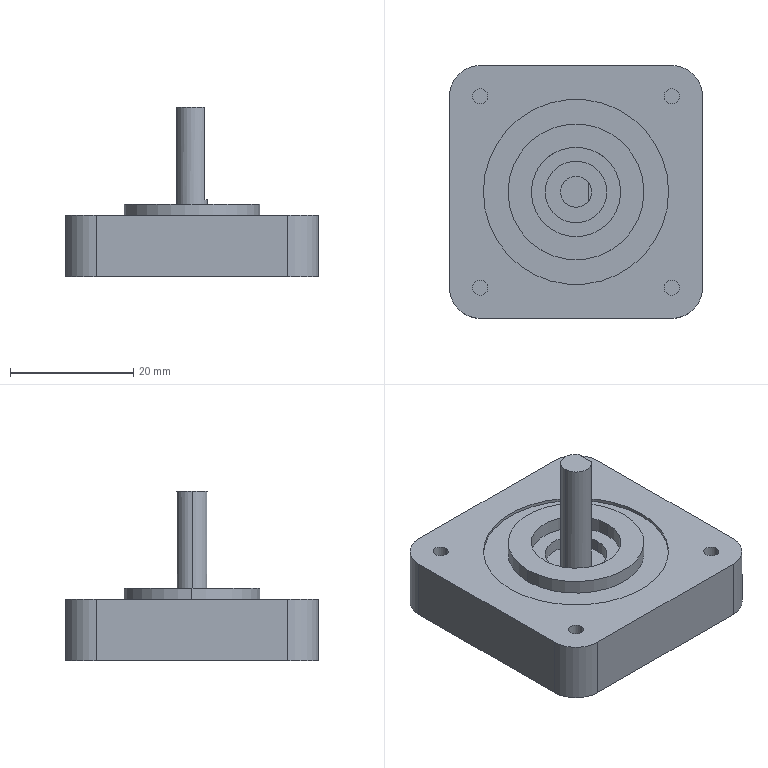Part | SolidWorks | features BaseBody 1 | 1 solid | 39 faces | box 41 x 41 x 27.5 mm | volume 16881 mm3 | cylinder 22 | plane 17 | commonest cylinder face diameters 2.459 x8 10 x6 5 x2 14.5 x2 22 x2 30 x2
STEP:
#1=CARTESIAN_POINT('',(-2.739,-8.029,6.));
#2=VERTEX_POINT('',#1);
#3=CARTESIAN_POINT('',(-0.2798,-8.029,6.));
#4=VERTEX_POINT('',#3);
#5=CARTESIAN_POINT('',(-1.509,-8.029,6.));
#6=DIRECTION('',(0.,0.,1.));
#7=DIRECTION('',(1.,0.,0.));
#8=AXIS2_PLACEMENT_3D('',#5,#6,#7);
#9=CIRCLE('',#8,1.23);
#10=EDGE_CURVE('',#2,#4,#9,.T.);
#11=ORIENTED_EDGE('',*,*,#10,.F.);
#12=CARTESIAN_POINT('',(-2.739,-8.029,10.));
#13=VERTEX_POINT('',#12);
#14=CARTESIAN_POINT('',(-2.739,-8.029,8.));
#15=DIRECTION('',(0.,0.,1.));
#16=VECTOR('',#15,1000.);
#17=LINE('',#14,#16);
#18=EDGE_CURVE('',#2,#13,#17,.T.);
#19=ORIENTED_EDGE('',*,*,#18,.T.);
#20=CARTESIAN_POINT('',(-0.2798,-8.029,10.));
#21=VERTEX_POINT('',#20);
#22=CARTESIAN_POINT('',(-1.509,-8.029,10.));
#23=DIRECTION('',(0.,0.,-1.));
#24=DIRECTION('',(1.,0.,0.));
#25=AXIS2_PLACEMENT_3D('',#22,#23,#24);
#26=CIRCLE('',#25,1.23);
#27=EDGE_CURVE('',#21,#13,#26,.T.);
#28=ORIENTED_EDGE('',*,*,#27,.F.);
#29=CARTESIAN_POINT('',(-0.2798,-8.029,8.));
#30=DIRECTION('',(0.,0.,1.));
#31=VECTOR('',#30,1000.);
#32=LINE('',#29,#31);
#33=EDGE_CURVE('',#4,#21,#32,.T.);
#34=ORIENTED_EDGE('',*,*,#33,.F.);
#35=EDGE_LOOP('',(#11,#19,#28,#34));
#36=FACE_OUTER_BOUND('',#35,.T.);
#37=CARTESIAN_POINT('',(-1.509,-8.029,8.));
#38=DIRECTION('',(0.,0.,1.));
#39=DIRECTION('',(1.,0.,0.));
#40=AXIS2_PLACEMENT_3D('',#37,#38,#39);
#41=CYLINDRICAL_SURFACE('',#40,1.23);
#42=ADVANCED_FACE('',(#36),#41,.F.);
#43=CARTESIAN_POINT('',(-33.739,-8.029,6.));
#44=VERTEX_POINT('',#43);
#45=CARTESIAN_POINT('',(-31.28,-8.029,6.));
#46=VERTEX_POINT('',#45);
#47=CARTESIAN_POINT('',(-32.509,-8.029,6.));
#48=DIRECTION('',(0.,0.,1.));
#49=DIRECTION('',(1.,0.,0.));
#50=AXIS2_PLACEMENT_3D('',#47,#48,#49);
#51=CIRCLE('',#50,1.23);
#52=EDGE_CURVE('',#44,#46,#51,.T.);
#53=ORIENTED_EDGE('',*,*,#52,.F.);
#54=CARTESIAN_POINT('',(-33.739,-8.029,10.));
#55=VERTEX_POINT('',#54);
#56=CARTESIAN_POINT('',(-33.739,-8.029,8.));
#57=DIRECTION('',(0.,0.,1.));
#58=VECTOR('',#57,1000.);
#59=LINE('',#56,#58);
#60=EDGE_CURVE('',#44,#55,#59,.T.);
#61=ORIENTED_EDGE('',*,*,#60,.T.);
#62=CARTESIAN_POINT('',(-31.28,-8.029,10.));
#63=VERTEX_POINT('',#62);
#64=CARTESIAN_POINT('',(-32.509,-8.029,10.));
#65=DIRECTION('',(0.,0.,-1.));
#66=DIRECTION('',(1.,0.,0.));
#67=AXIS2_PLACEMENT_3D('',#64,#65,#66);
#68=CIRCLE('',#67,1.23);
#69=EDGE_CURVE('',#63,#55,#68,.T.);
#70=ORIENTED_EDGE('',*,*,#69,.F.);
#71=CARTESIAN_POINT('',(-31.28,-8.029,8.));
#72=DIRECTION('',(0.,0.,1.));
#73=VECTOR('',#72,1000.);
#74=LINE('',#71,#73);
#75=EDGE_CURVE('',#46,#63,#74,.T.);
#76=ORIENTED_EDGE('',*,*,#75,.F.);
#77=EDGE_LOOP('',(#53,#61,#70,#76));
#78=FACE_OUTER_BOUND('',#77,.T.);
#79=CARTESIAN_POINT('',(-32.509,-8.029,8.));
#80=DIRECTION('',(0.,0.,1.));
#81=DIRECTION('',(1.,0.,0.));
#82=AXIS2_PLACEMENT_3D('',#79,#80,#81);
#83=CYLINDRICAL_SURFACE('',#82,1.23);
#84=ADVANCED_FACE('',(#78),#83,.F.);
#85=CARTESIAN_POINT('',(-33.739,22.971,6.));
#86=VERTEX_POINT('',#85);
#87=CARTESIAN_POINT('',(-31.28,22.971,6.));
#88=VERTEX_POINT('',#87);
#89=CARTESIAN_POINT('',(-32.509,22.971,6.));
#90=DIRECTION('',(0.,0.,1.));
#91=DIRECTION('',(1.,0.,0.));
#92=AXIS2_PLACEMENT_3D('',#89,#90,#91);
#93=CIRCLE('',#92,1.23);
#94=EDGE_CURVE('',#86,#88,#93,.T.);
#95=ORIENTED_EDGE('',*,*,#94,.F.);
#96=CARTESIAN_POINT('',(-33.739,22.971,10.));
#97=VERTEX_POINT('',#96);
#98=CARTESIAN_POINT('',(-33.739,22.971,8.));
#99=DIRECTION('',(0.,0.,1.));
#100=VECTOR('',#99,1000.);
#101=LINE('',#98,#100);
#102=EDGE_CURVE('',#86,#97,#101,.T.);
#103=ORIENTED_EDGE('',*,*,#102,.T.);
#104=CARTESIAN_POINT('',(-31.28,22.971,10.));
#105=VERTEX_POINT('',#104);
#106=CARTESIAN_POINT('',(-32.509,22.971,10.));
#107=DIRECTION('',(0.,0.,-1.));
#108=DIRECTION('',(1.,0.,0.));
#109=AXIS2_PLACEMENT_3D('',#106,#107,#108);
#110=CIRCLE('',#109,1.23);
#111=EDGE_CURVE('',#105,#97,#110,.T.);
#112=ORIENTED_EDGE('',*,*,#111,.F.);
#113=CARTESIAN_POINT('',(-31.28,22.971,8.));
#114=DIRECTION('',(0.,0.,1.));
#115=VECTOR('',#114,1000.);
#116=LINE('',#113,#115);
#117=EDGE_CURVE('',#88,#105,#116,.T.);
#118=ORIENTED_EDGE('',*,*,#117,.F.);
#119=EDGE_LOOP('',(#95,#103,#112,#118));
#120=FACE_OUTER_BOUND('',#119,.T.);
#121=CARTESIAN_POINT('',(-32.509,22.971,8.));
#122=DIRECTION('',(0.,0.,1.));
#123=DIRECTION('',(1.,0.,0.));
#124=AXIS2_PLACEMENT_3D('',#121,#122,#123);
#125=CYLINDRICAL_SURFACE('',#124,1.23);
#126=ADVANCED_FACE('',(#120),#125,.F.);
#127=CARTESIAN_POINT('',(-2.739,22.971,6.));
#128=VERTEX_POINT('',#127);
#129=CARTESIAN_POINT('',(-0.2798,22.971,6.));
#130=VERTEX_POINT('',#129);
#131=CARTESIAN_POINT('',(-1.509,22.971,6.));
#132=DIRECTION('',(0.,0.,1.));
#133=DIRECTION('',(1.,0.,0.));
#134=AXIS2_PLACEMENT_3D('',#131,#132,#133);
#135=CIRCLE('',#134,1.23);
#136=EDGE_CURVE('',#128,#130,#135,.T.);
#137=ORIENTED_EDGE('',*,*,#136,.F.);
#138=CARTESIAN_POINT('',(-2.739,22.971,10.));
#139=VERTEX_POINT('',#138);
#140=CARTESIAN_POINT('',(-2.739,22.971,8.));
#141=DIRECTION('',(0.,0.,1.));
#142=VECTOR('',#141,1000.);
#143=LINE('',#140,#142);
#144=EDGE_CURVE('',#128,#139,#143,.T.);
#145=ORIENTED_EDGE('',*,*,#144,.T.);
#146=CARTESIAN_POINT('',(-0.2798,22.971,10.));
#147=VERTEX_POINT('',#146);
#148=CARTESIAN_POINT('',(-1.509,22.971,10.));
#149=DIRECTION('',(0.,0.,-1.));
#150=DIRECTION('',(1.,0.,0.));
#151=AXIS2_PLACEMENT_3D('',#148,#149,#150);
#152=CIRCLE('',#151,1.23);
#153=EDGE_CURVE('',#147,#139,#152,.T.);
#154=ORIENTED_EDGE('',*,*,#153,.F.);
#155=CARTESIAN_POINT('',(-0.2798,22.971,8.));
#156=DIRECTION('',(0.,0.,1.));
#157=VECTOR('',#156,1000.);
#158=LINE('',#155,#157);
#159=EDGE_CURVE('',#130,#147,#158,.T.);
#160=ORIENTED_EDGE('',*,*,#159,.F.);
#161=EDGE_LOOP('',(#137,#145,#154,#160));
#162=FACE_OUTER_BOUND('',#161,.T.);
#163=CARTESIAN_POINT('',(-1.509,22.971,8.));
#164=DIRECTION('',(0.,0.,1.));
#165=DIRECTION('',(1.,0.,0.));
#166=AXIS2_PLACEMENT_3D('',#163,#164,#165);
#167=CYLINDRICAL_SURFACE('',#166,1.23);
#168=ADVANCED_FACE('',(#162),#167,.F.);
#169=CARTESIAN_POINT('',(-2.009,7.471,10.));
#170=VERTEX_POINT('',#169);
#171=CARTESIAN_POINT('',(-32.009,7.471,10.));
#172=VERTEX_POINT('',#171);
#173=CARTESIAN_POINT('',(-17.009,7.471,10.));
#174=DIRECTION('',(0.,0.,-1.));
#175=DIRECTION('',(-1.,0.,0.));
#176=AXIS2_PLACEMENT_3D('',#173,#174,#175);
#177=CIRCLE('',#176,15.);
#178=EDGE_CURVE('',#170,#172,#177,.T.);
#179=ORIENTED_EDGE('',*,*,#178,.F.);
#180=CARTESIAN_POINT('',(-2.009,7.471,9.5));
#181=VERTEX_POINT('',#180);
#182=CARTESIAN_POINT('',(-2.009,7.471,10.));
#183=DIRECTION('',(0.,0.,-1.));
#184=VECTOR('',#183,1000.);
#185=LINE('',#182,#184);
#186=EDGE_CURVE('',#170,#181,#185,.T.);
#187=ORIENTED_EDGE('',*,*,#186,.T.);
#188=CARTESIAN_POINT('',(-32.009,7.471,9.5));
#189=VERTEX_POINT('',#188);
#190=CARTESIAN_POINT('',(-17.009,7.471,9.5));
#191=DIRECTION('',(0.,0.,1.));
#192=DIRECTION('',(-1.,0.,0.));
#193=AXIS2_PLACEMENT_3D('',#190,#191,#192);
#194=CIRCLE('',#193,15.);
#195=EDGE_CURVE('',#189,#181,#194,.T.);
#196=ORIENTED_EDGE('',*,*,#195,.F.);
#197=CARTESIAN_POINT('',(-32.009,7.471,10.));
#198=DIRECTION('',(0.,0.,-1.));
#199=VECTOR('',#198,1000.);
#200=LINE('',#197,#199);
#201=EDGE_CURVE('',#172,#189,#200,.T.);
#202=ORIENTED_EDGE('',*,*,#201,.F.);
#203=EDGE_LOOP('',(#179,#187,#196,#202));
#204=FACE_OUTER_BOUND('',#203,.T.);
#205=CARTESIAN_POINT('',(-17.009,7.471,10.));
#206=DIRECTION('',(0.,0.,-1.));
#207=DIRECTION('',(-1.,0.,0.));
#208=AXIS2_PLACEMENT_3D('',#205,#206,#207);
#209=CYLINDRICAL_SURFACE('',#208,15.);
#210=ADVANCED_FACE('',(#204),#209,.F.);
#211=CARTESIAN_POINT('',(-6.009,7.471,9.5));
#212=VERTEX_POINT('',#211);
#213=CARTESIAN_POINT('',(-28.009,7.471,9.5));
#214=VERTEX_POINT('',#213);
#215=CARTESIAN_POINT('',(-17.009,7.471,9.5));
#216=DIRECTION('',(0.,0.,1.));
#217=DIRECTION('',(1.,0.,0.));
#218=AXIS2_PLACEMENT_3D('',#215,#216,#217);
#219=CIRCLE('',#218,11.);
#220=EDGE_CURVE('',#212,#214,#219,.T.);
#221=ORIENTED_EDGE('',*,*,#220,.T.);
#222=CARTESIAN_POINT('',(-28.009,7.471,11.8));
#223=VERTEX_POINT('',#222);
#224=CARTESIAN_POINT('',(-28.009,7.471,9.5));
#225=DIRECTION('',(0.,0.,1.));
#226=VECTOR('',#225,1000.);
#227=LINE('',#224,#226);
#228=EDGE_CURVE('',#214,#223,#227,.T.);
#229=ORIENTED_EDGE('',*,*,#228,.T.);
#230=CARTESIAN_POINT('',(-6.009,7.471,11.8));
#231=VERTEX_POINT('',#230);
#232=CARTESIAN_POINT('',(-17.009,7.471,11.8));
#233=DIRECTION('',(0.,0.,-1.));
#234=DIRECTION('',(1.,0.,0.));
#235=AXIS2_PLACEMENT_3D('',#232,#233,#234);
#236=CIRCLE('',#235,11.);
#237=EDGE_CURVE('',#223,#231,#236,.T.);
#238=ORIENTED_EDGE('',*,*,#237,.T.);
#239=CARTESIAN_POINT('',(-6.009,7.471,9.5));
#240=DIRECTION('',(0.,0.,1.));
#241=VECTOR('',#240,1000.);
#242=LINE('',#239,#241);
#243=EDGE_CURVE('',#212,#231,#242,.T.);
#244=ORIENTED_EDGE('',*,*,#243,.F.);
#245=EDGE_LOOP('',(#221,#229,#238,#244));
#246=FACE_OUTER_BOUND('',#245,.T.);
#247=CARTESIAN_POINT('',(-17.009,7.471,9.5));
#248=DIRECTION('',(0.,0.,1.));
#249=DIRECTION('',(1.,0.,0.));
#250=AXIS2_PLACEMENT_3D('',#247,#248,#249);
#251=CYLINDRICAL_SURFACE('',#250,11.);
#252=ADVANCED_FACE('',(#246),#251,.T.);
#253=CARTESIAN_POINT('',(-24.259,7.471,9.5));
#254=VERTEX_POINT('',#253);
#255=CARTESIAN_POINT('',(-9.759,7.471,9.5));
#256=VERTEX_POINT('',#255);
#257=CARTESIAN_POINT('',(-17.009,7.471,9.5));
#258=DIRECTION('',(0.,0.,1.));
#259=DIRECTION('',(1.,0.,0.));
#260=AXIS2_PLACEMENT_3D('',#257,#258,#259);
#261=CIRCLE('',#260,7.25);
#262=EDGE_CURVE('',#254,#256,#261,.T.);
#263=ORIENTED_EDGE('',*,*,#262,.F.);
#264=CARTESIAN_POINT('',(-24.259,7.471,11.8));
#265=VERTEX_POINT('',#264);
#266=CARTESIAN_POINT('',(-24.259,7.471,10.65));
#267=DIRECTION('',(0.,0.,1.));
#268=VECTOR('',#267,1000.);
#269=LINE('',#266,#268);
#270=EDGE_CURVE('',#254,#265,#269,.T.);
#271=ORIENTED_EDGE('',*,*,#270,.T.);
#272=CARTESIAN_POINT('',(-9.759,7.471,11.8));
#273=VERTEX_POINT('',#272);
#274=CARTESIAN_POINT('',(-17.009,7.471,11.8));
#275=DIRECTION('',(0.,0.,1.));
#276=DIRECTION('',(1.,0.,0.));
#277=AXIS2_PLACEMENT_3D('',#274,#275,#276);
#278=CIRCLE('',#277,7.25);
#279=EDGE_CURVE('',#265,#273,#278,.T.);
#280=ORIENTED_EDGE('',*,*,#279,.T.);
#281=CARTESIAN_POINT('',(-9.759,7.471,10.65));
#282=DIRECTION('',(0.,0.,1.));
#283=VECTOR('',#282,1000.);
#284=LINE('',#281,#283);
#285=EDGE_CURVE('',#256,#273,#284,.T.);
#286=ORIENTED_EDGE('',*,*,#285,.F.);
#287=EDGE_LOOP('',(#263,#271,#280,#286));
#288=FACE_OUTER_BOUND('',#287,.T.);
#289=CARTESIAN_POINT('',(-17.009,7.471,10.65));
#290=DIRECTION('',(0.,0.,1.));
#291=DIRECTION('',(1.,0.,0.));
#292=AXIS2_PLACEMENT_3D('',#289,#290,#291);
#293=CYLINDRICAL_SURFACE('',#292,7.25);
#294=ADVANCED_FACE('',(#288),#293,.F.);
#295=CARTESIAN_POINT('',(-22.009,7.471,7.5));
#296=VERTEX_POINT('',#295);
#297=CARTESIAN_POINT('',(-12.009,7.471,7.5));
#298=VERTEX_POINT('',#297);
#299=CARTESIAN_POINT('',(-17.009,7.471,7.5));
#300=DIRECTION('',(0.,0.,1.));
#301=DIRECTION('',(1.,0.,0.));
#302=AXIS2_PLACEMENT_3D('',#299,#300,#301);
#303=CIRCLE('',#302,5.);
#304=EDGE_CURVE('',#296,#298,#303,.T.);
#305=ORIENTED_EDGE('',*,*,#304,.F.);
#306=CARTESIAN_POINT('',(-22.009,7.471,9.5));
#307=VERTEX_POINT('',#306);
#308=CARTESIAN_POINT('',(-22.009,7.471,8.75));
#309=DIRECTION('',(0.,0.,1.));
#310=VECTOR('',#309,1000.);
#311=LINE('',#308,#310);
#312=EDGE_CURVE('',#296,#307,#311,.T.);
#313=ORIENTED_EDGE('',*,*,#312,.T.);
#314=CARTESIAN_POINT('',(-12.009,7.471,9.5));
#315=VERTEX_POINT('',#314);
#316=CARTESIAN_POINT('',(-17.009,7.471,9.5));
#317=DIRECTION('',(0.,0.,-1.));
#318=DIRECTION('',(1.,0.,0.));
#319=AXIS2_PLACEMENT_3D('',#316,#317,#318);
#320=CIRCLE('',#319,5.);
#321=EDGE_CURVE('',#315,#307,#320,.T.);
#322=ORIENTED_EDGE('',*,*,#321,.F.);
#323=CARTESIAN_POINT('',(-12.009,7.471,8.75));
#324=DIRECTION('',(0.,0.,1.));
#325=VECTOR('',#324,1000.);
#326=LINE('',#323,#325);
#327=EDGE_CURVE('',#298,#315,#326,.T.);
#328=ORIENTED_EDGE('',*,*,#327,.F.);
#329=EDGE_LOOP('',(#305,#313,#322,#328));
#330=FACE_OUTER_BOUND('',#329,.T.);
#331=CARTESIAN_POINT('',(-17.009,7.471,8.75));
#332=DIRECTION('',(0.,0.,1.));
#333=DIRECTION('',(1.,0.,0.));
#334=AXIS2_PLACEMENT_3D('',#331,#332,#333);
#335=CYLINDRICAL_SURFACE('',#334,5.);
#336=ADVANCED_FACE('',(#330),#335,.F.);
#337=CARTESIAN_POINT('',(-19.509,7.471,7.5));
#338=VERTEX_POINT('',#337);
#339=CARTESIAN_POINT('',(-14.509,7.471,7.5));
#340=VERTEX_POINT('',#339);
#341=CARTESIAN_POINT('',(-17.009,7.471,7.5));
#342=DIRECTION('',(0.,0.,-1.));
#343=DIRECTION('',(1.,0.,0.));
#344=AXIS2_PLACEMENT_3D('',#341,#342,#343);
#345=CIRCLE('',#344,2.5);
#346=EDGE_CURVE('',#338,#340,#345,.T.);
#347=ORIENTED_EDGE('',*,*,#346,.F.);
#348=CARTESIAN_POINT('',(-19.509,7.471,27.5));
#349=VERTEX_POINT('',#348);
#350=CARTESIAN_POINT('',(-19.509,7.471,7.5));
#351=DIRECTION('',(0.,0.,1.));
#352=VECTOR('',#351,1000.);
#353=LINE('',#350,#352);
#354=EDGE_CURVE('',#338,#349,#353,.T.);
#355=ORIENTED_EDGE('',*,*,#354,.T.);
#356=CARTESIAN_POINT('',(-15.009,8.971,27.5));
#357=VERTEX_POINT('',#356);
#358=CARTESIAN_POINT('',(-17.009,7.471,27.5));
#359=DIRECTION('',(0.,0.,-1.));
#360=DIRECTION('',(1.,0.,0.));
#361=AXIS2_PLACEMENT_3D('',#358,#359,#360);
#362=CIRCLE('',#361,2.5);
#363=EDGE_CURVE('',#349,#357,#362,.T.);
#364=ORIENTED_EDGE('',*,*,#363,.T.);
#365=CARTESIAN_POINT('',(-15.009,8.971,12.5));
#366=VERTEX_POINT('',#365);
#367=CARTESIAN_POINT('',(-15.009,8.971,7.5));
#368=DIRECTION('',(0.,0.,-1.));
#369=VECTOR('',#368,1000.);
#370=LINE('',#367,#369);
#371=EDGE_CURVE('',#357,#366,#370,.T.);
#372=ORIENTED_EDGE('',*,*,#371,.T.);
#373=CARTESIAN_POINT('',(-14.509,7.471,12.5));
#374=VERTEX_POINT('',#373);
#375=CARTESIAN_POINT('',(-17.009,7.471,12.5));
#376=DIRECTION('',(0.,0.,-1.));
#377=DIRECTION('',(1.,0.,0.));
#378=AXIS2_PLACEMENT_3D('',#375,#376,#377);
#379=CIRCLE('',#378,2.5);
#380=EDGE_CURVE('',#366,#374,#379,.T.);
#381=ORIENTED_EDGE('',*,*,#380,.T.);
#382=CARTESIAN_POINT('',(-14.509,7.471,7.5));
#383=DIRECTION('',(0.,0.,1.));
#384=VECTOR('',#383,1000.);
#385=LINE('',#382,#384);
#386=EDGE_CURVE('',#340,#374,#385,.T.);
#387=ORIENTED_EDGE('',*,*,#386,.F.);
#388=EDGE_LOOP('',(#347,#355,#364,#372,#381,#387));
#389=FACE_OUTER_BOUND('',#388,.T.);
#390=CARTESIAN_POINT('',(-17.009,7.471,7.5));
#391=DIRECTION('',(0.,0.,1.));
#392=DIRECTION('',(1.,0.,0.));
#393=AXIS2_PLACEMENT_3D('',#390,#391,#392);
#394=CYLINDRICAL_SURFACE('',#393,2.5);
#395=ADVANCED_FACE('',(#389),#394,.T.);
#396=CARTESIAN_POINT('',(-37.509,22.971,0.));
#397=VERTEX_POINT('',#396);
#398=CARTESIAN_POINT('',(-37.509,-8.029,0.));
#399=VERTEX_POINT('',#398);
#400=CARTESIAN_POINT('',(-37.509,7.471,0.));
#401=DIRECTION('',(0.,-1.,0.));
#402=VECTOR('',#401,1000.);
#403=LINE('',#400,#402);
#404=EDGE_CURVE('',#397,#399,#403,.T.);
#405=ORIENTED_EDGE('',*,*,#404,.F.);
#406=CARTESIAN_POINT('',(-32.509,27.971,0.));
#407=VERTEX_POINT('',#406);
#408=CARTESIAN_POINT('',(-32.509,22.971,0.));
#409=DIRECTION('',(0.,0.,1.));
#410=DIRECTION('',(1.,0.,0.));
#411=AXIS2_PLACEMENT_3D('',#408,#409,#410);
#412=CIRCLE('',#411,5.);
#413=EDGE_CURVE('',#407,#397,#412,.T.);
#414=ORIENTED_EDGE('',*,*,#413,.F.);
#415=CARTESIAN_POINT('',(-1.509,27.971,0.));
#416=VERTEX_POINT('',#415);
#417=CARTESIAN_POINT('',(-17.009,27.971,0.));
#418=DIRECTION('',(-1.,0.,0.));
#419=VECTOR('',#418,1000.);
#420=LINE('',#417,#419);
#421=EDGE_CURVE('',#416,#407,#420,.T.);
#422=ORIENTED_EDGE('',*,*,#421,.F.);
#423=CARTESIAN_POINT('',(3.491,22.971,0.));
#424=VERTEX_POINT('',#423);
#425=CARTESIAN_POINT('',(-1.509,22.971,0.));
#426=DIRECTION('',(0.,0.,1.));
#427=DIRECTION('',(1.,0.,0.));
#428=AXIS2_PLACEMENT_3D('',#425,#426,#427);
#429=CIRCLE('',#428,5.);
#430=EDGE_CURVE('',#424,#416,#429,.T.);
#431=ORIENTED_EDGE('',*,*,#430,.F.);
#432=CARTESIAN_POINT('',(3.491,-8.029,0.));
#433=VERTEX_POINT('',#432);
#434=CARTESIAN_POINT('',(3.491,7.471,0.));
#435=DIRECTION('',(0.,1.,0.));
#436=VECTOR('',#435,1000.);
#437=LINE('',#434,#436);
#438=EDGE_CURVE('',#433,#424,#437,.T.);
#439=ORIENTED_EDGE('',*,*,#438,.F.);
#440=CARTESIAN_POINT('',(-1.509,-13.029,0.));
#441=VERTEX_POINT('',#440);
#442=CARTESIAN_POINT('',(-1.509,-8.029,0.));
#443=DIRECTION('',(0.,0.,1.));
#444=DIRECTION('',(1.,0.,0.));
#445=AXIS2_PLACEMENT_3D('',#442,#443,#444);
#446=CIRCLE('',#445,5.);
#447=EDGE_CURVE('',#441,#433,#446,.T.);
#448=ORIENTED_EDGE('',*,*,#447,.F.);
#449=CARTESIAN_POINT('',(-32.509,-13.029,0.));
#450=VERTEX_POINT('',#449);
#451=CARTESIAN_POINT('',(-17.009,-13.029,0.));
#452=DIRECTION('',(1.,0.,0.));
#453=VECTOR('',#452,1000.);
#454=LINE('',#451,#453);
#455=EDGE_CURVE('',#450,#441,#454,.T.);
#456=ORIENTED_EDGE('',*,*,#455,.F.);
#457=CARTESIAN_POINT('',(-32.509,-8.029,0.));
#458=DIRECTION('',(0.,0.,1.));
#459=DIRECTION('',(1.,0.,0.));
#460=AXIS2_PLACEMENT_3D('',#457,#458,#459);
#461=CIRCLE('',#460,5.);
#462=EDGE_CURVE('',#399,#450,#461,.T.);
#463=ORIENTED_EDGE('',*,*,#462,.F.);
#464=EDGE_LOOP('',(#405,#414,#422,#431,#439,#448,#456,#463));
#465=FACE_OUTER_BOUND('',#464,.T.);
#466=CARTESIAN_POINT('',(-17.009,7.471,0.));
#467=DIRECTION('',(0.,0.,1.));
#468=DIRECTION('',(1.,0.,0.));
#469=AXIS2_PLACEMENT_3D('',#466,#467,#468);
#470=PLANE('',#469);
#471=ADVANCED_FACE('',(#465),#470,.F.);
#472=ORIENTED_EDGE('',*,*,#462,.T.);
#473=CARTESIAN_POINT('',(-32.509,-13.029,10.));
#474=VERTEX_POINT('',#473);
#475=CARTESIAN_POINT('',(-32.509,-13.029,0.));
#476=DIRECTION('',(0.,0.,1.));
#477=VECTOR('',#476,1000.);
#478=LINE('',#475,#477);
#479=EDGE_CURVE('',#450,#474,#478,.T.);
#480=ORIENTED_EDGE('',*,*,#479,.T.);
#481=CARTESIAN_POINT('',(-37.509,-8.029,10.));
#482=VERTEX_POINT('',#481);
#483=CARTESIAN_POINT('',(-32.509,-8.029,10.));
#484=DIRECTION('',(0.,0.,-1.));
#485=DIRECTION('',(1.,0.,0.));
#486=AXIS2_PLACEMENT_3D('',#483,#484,#485);
#487=CIRCLE('',#486,5.);
#488=EDGE_CURVE('',#474,#482,#487,.T.);
#489=ORIENTED_EDGE('',*,*,#488,.T.);
#490=CARTESIAN_POINT('',(-37.509,-8.029,0.));
#491=DIRECTION('',(0.,0.,-1.));
#492=VECTOR('',#491,1000.);
#493=LINE('',#490,#492);
#494=EDGE_CURVE('',#482,#399,#493,.T.);
#495=ORIENTED_EDGE('',*,*,#494,.T.);
#496=EDGE_LOOP('',(#472,#480,#489,#495));
#497=FACE_OUTER_BOUND('',#496,.T.);
#498=CARTESIAN_POINT('',(-32.509,-8.029,0.));
#499=DIRECTION('',(0.,0.,1.));
#500=DIRECTION('',(1.,0.,0.));
#501=AXIS2_PLACEMENT_3D('',#498,#499,#500);
#502=CYLINDRICAL_SURFACE('',#501,5.);
#503=ADVANCED_FACE('',(#497),#502,.T.);
#504=CARTESIAN_POINT('',(-37.509,22.971,10.));
#505=VERTEX_POINT('',#504);
#506=CARTESIAN_POINT('',(-37.509,22.971,0.));
#507=DIRECTION('',(0.,0.,-1.));
#508=VECTOR('',#507,1000.);
#509=LINE('',#506,#508);
#510=EDGE_CURVE('',#505,#397,#509,.T.);
#511=ORIENTED_EDGE('',*,*,#510,.T.);
#512=ORIENTED_EDGE('',*,*,#404,.T.);
#513=ORIENTED_EDGE('',*,*,#494,.F.);
#514=CARTESIAN_POINT('',(-37.509,-13.029,10.));
#515=DIRECTION('',(0.,1.,0.));
#516=VECTOR('',#515,1000.);
#517=LINE('',#514,#516);
#518=EDGE_CURVE('',#482,#505,#517,.T.);
#519=ORIENTED_EDGE('',*,*,#518,.T.);
#520=EDGE_LOOP('',(#511,#512,#513,#519));
#521=FACE_OUTER_BOUND('',#520,.T.);
#522=CARTESIAN_POINT('',(-37.509,-13.029,0.));
#523=DIRECTION('',(-1.,0.,0.));
#524=DIRECTION('',(0.,0.,1.));
#525=AXIS2_PLACEMENT_3D('',#522,#523,#524);
#526=PLANE('',#525);
#527=ADVANCED_FACE('',(#521),#526,.T.);
#528=ORIENTED_EDGE('',*,*,#413,.T.);
#529=ORIENTED_EDGE('',*,*,#510,.F.);
#530=CARTESIAN_POINT('',(-32.509,27.971,10.));
#531=VERTEX_POINT('',#530);
#532=CARTESIAN_POINT('',(-32.509,22.971,10.));
#533=DIRECTION('',(0.,0.,-1.));
#534=DIRECTION('',(1.,0.,0.));
#535=AXIS2_PLACEMENT_3D('',#532,#533,#534);
#536=CIRCLE('',#535,5.);
#537=EDGE_CURVE('',#505,#531,#536,.T.);
#538=ORIENTED_EDGE('',*,*,#537,.T.);
#539=CARTESIAN_POINT('',(-32.509,27.971,0.));
#540=DIRECTION('',(0.,0.,-1.));
#541=VECTOR('',#540,1000.);
#542=LINE('',#539,#541);
#543=EDGE_CURVE('',#531,#407,#542,.T.);
#544=ORIENTED_EDGE('',*,*,#543,.T.);
#545=EDGE_LOOP('',(#528,#529,#538,#544));
#546=FACE_OUTER_BOUND('',#545,.T.);
#547=CARTESIAN_POINT('',(-32.509,22.971,0.));
#548=DIRECTION('',(0.,0.,1.));
#549=DIRECTION('',(1.,0.,0.));
#550=AXIS2_PLACEMENT_3D('',#547,#548,#549);
#551=CYLINDRICAL_SURFACE('',#550,5.);
#552=ADVANCED_FACE('',(#546),#551,.T.);
#553=ORIENTED_EDGE('',*,*,#543,.F.);
#554=CARTESIAN_POINT('',(-1.509,27.971,10.));
#555=VERTEX_POINT('',#554);
#556=CARTESIAN_POINT('',(-37.509,27.971,10.));
#557=DIRECTION('',(1.,0.,0.));
#558=VECTOR('',#557,1000.);
#559=LINE('',#556,#558);
#560=EDGE_CURVE('',#531,#555,#559,.T.);
#561=ORIENTED_EDGE('',*,*,#560,.T.);
#562=CARTESIAN_POINT('',(-1.509,27.971,0.));
#563=DIRECTION('',(0.,0.,-1.));
#564=VECTOR('',#563,1000.);
#565=LINE('',#562,#564);
#566=EDGE_CURVE('',#555,#416,#565,.T.);
#567=ORIENTED_EDGE('',*,*,#566,.T.);
#568=ORIENTED_EDGE('',*,*,#421,.T.);
#569=EDGE_LOOP('',(#553,#561,#567,#568));
#570=FACE_OUTER_BOUND('',#569,.T.);
#571=CARTESIAN_POINT('',(-37.509,27.971,0.));
#572=DIRECTION('',(0.,1.,0.));
#573=DIRECTION('',(0.,0.,1.));
#574=AXIS2_PLACEMENT_3D('',#571,#572,#573);
#575=PLANE('',#574);
#576=ADVANCED_FACE('',(#570),#575,.T.);
#577=ORIENTED_EDGE('',*,*,#430,.T.);
#578=ORIENTED_EDGE('',*,*,#566,.F.);
#579=CARTESIAN_POINT('',(3.491,22.971,10.));
#580=VERTEX_POINT('',#579);
#581=CARTESIAN_POINT('',(-1.509,22.971,10.));
#582=DIRECTION('',(0.,0.,-1.));
#583=DIRECTION('',(1.,0.,0.));
#584=AXIS2_PLACEMENT_3D('',#581,#582,#583);
#585=CIRCLE('',#584,5.);
#586=EDGE_CURVE('',#555,#580,#585,.T.);
#587=ORIENTED_EDGE('',*,*,#586,.T.);
#588=CARTESIAN_POINT('',(3.491,22.971,0.));
#589=DIRECTION('',(0.,0.,-1.));
#590=VECTOR('',#589,1000.);
#591=LINE('',#588,#590);
#592=EDGE_CURVE('',#580,#424,#591,.T.);
#593=ORIENTED_EDGE('',*,*,#592,.T.);
#594=EDGE_LOOP('',(#577,#578,#587,#593));
#595=FACE_OUTER_BOUND('',#594,.T.);
#596=CARTESIAN_POINT('',(-1.509,22.971,0.));
#597=DIRECTION('',(0.,0.,1.));
#598=DIRECTION('',(1.,0.,0.));
#599=AXIS2_PLACEMENT_3D('',#596,#597,#598);
#600=CYLINDRICAL_SURFACE('',#599,5.);
#601=ADVANCED_FACE('',(#595),#600,.T.);
#602=ORIENTED_EDGE('',*,*,#592,.F.);
#603=CARTESIAN_POINT('',(3.491,-8.029,10.));
#604=VERTEX_POINT('',#603);
#605=CARTESIAN_POINT('',(3.491,27.971,10.));
#606=DIRECTION('',(0.,-1.,0.));
#607=VECTOR('',#606,1000.);
#608=LINE('',#605,#607);
#609=EDGE_CURVE('',#580,#604,#608,.T.);
#610=ORIENTED_EDGE('',*,*,#609,.T.);
#611=CARTESIAN_POINT('',(3.491,-8.029,0.));
#612=DIRECTION('',(0.,0.,-1.));
#613=VECTOR('',#612,1000.);
#614=LINE('',#611,#613);
#615=EDGE_CURVE('',#604,#433,#614,.T.);
#616=ORIENTED_EDGE('',*,*,#615,.T.);
#617=ORIENTED_EDGE('',*,*,#438,.T.);
#618=EDGE_LOOP('',(#602,#610,#616,#617));
#619=FACE_OUTER_BOUND('',#618,.T.);
#620=CARTESIAN_POINT('',(3.491,27.971,0.));
#621=DIRECTION('',(1.,0.,0.));
#622=DIRECTION('',(0.,0.,-1.));
#623=AXIS2_PLACEMENT_3D('',#620,#621,#622);
#624=PLANE('',#623);
#625=ADVANCED_FACE('',(#619),#624,.T.);
#626=ORIENTED_EDGE('',*,*,#447,.T.);
#627=ORIENTED_EDGE('',*,*,#615,.F.);
#628=CARTESIAN_POINT('',(-1.509,-13.029,10.));
#629=VERTEX_POINT('',#628);
#630=CARTESIAN_POINT('',(-1.509,-8.029,10.));
#631=DIRECTION('',(0.,0.,-1.));
#632=DIRECTION('',(1.,0.,0.));
#633=AXIS2_PLACEMENT_3D('',#630,#631,#632);
#634=CIRCLE('',#633,5.);
#635=EDGE_CURVE('',#604,#629,#634,.T.);
#636=ORIENTED_EDGE('',*,*,#635,.T.);
#637=CARTESIAN_POINT('',(-1.509,-13.029,0.));
#638=DIRECTION('',(0.,0.,-1.));
#639=VECTOR('',#638,1000.);
#640=LINE('',#637,#639);
#641=EDGE_CURVE('',#629,#441,#640,.T.);
#642=ORIENTED_EDGE('',*,*,#641,.T.);
#643=EDGE_LOOP('',(#626,#627,#636,#642));
#644=FACE_OUTER_BOUND('',#643,.T.);
#645=CARTESIAN_POINT('',(-1.509,-8.029,0.));
#646=DIRECTION('',(0.,0.,1.));
#647=DIRECTION('',(1.,0.,0.));
#648=AXIS2_PLACEMENT_3D('',#645,#646,#647);
#649=CYLINDRICAL_SURFACE('',#648,5.);
#650=ADVANCED_FACE('',(#644),#649,.T.);
#651=ORIENTED_EDGE('',*,*,#641,.F.);
#652=CARTESIAN_POINT('',(3.491,-13.029,10.));
#653=DIRECTION('',(-1.,0.,0.));
#654=VECTOR('',#653,1000.);
#655=LINE('',#652,#654);
#656=EDGE_CURVE('',#629,#474,#655,.T.);
#657=ORIENTED_EDGE('',*,*,#656,.T.);
#658=ORIENTED_EDGE('',*,*,#479,.F.);
#659=ORIENTED_EDGE('',*,*,#455,.T.);
#660=EDGE_LOOP('',(#651,#657,#658,#659));
#661=FACE_OUTER_BOUND('',#660,.T.);
#662=CARTESIAN_POINT('',(3.491,-13.029,0.));
#663=DIRECTION('',(0.,-1.,0.));
#664=DIRECTION('',(0.,0.,-1.));
#665=AXIS2_PLACEMENT_3D('',#662,#663,#664);
#666=PLANE('',#665);
#667=ADVANCED_FACE('',(#661),#666,.T.);
#668=ORIENTED_EDGE('',*,*,#27,.T.);
#669=CARTESIAN_POINT('',(-1.509,-8.029,10.));
#670=DIRECTION('',(0.,0.,-1.));
#671=DIRECTION('',(1.,0.,0.));
#672=AXIS2_PLACEMENT_3D('',#669,#670,#671);
#673=CIRCLE('',#672,1.23);
#674=EDGE_CURVE('',#13,#21,#673,.T.);
#675=ORIENTED_EDGE('',*,*,#674,.T.);
#676=EDGE_LOOP('',(#668,#675));
#677=FACE_BOUND('',#676,.T.);
#678=ORIENTED_EDGE('',*,*,#69,.T.);
#679=CARTESIAN_POINT('',(-32.509,-8.029,10.));
#680=DIRECTION('',(0.,0.,-1.));
#681=DIRECTION('',(1.,0.,0.));
#682=AXIS2_PLACEMENT_3D('',#679,#680,#681);
#683=CIRCLE('',#682,1.23);
#684=EDGE_CURVE('',#55,#63,#683,.T.);
#685=ORIENTED_EDGE('',*,*,#684,.T.);
#686=EDGE_LOOP('',(#678,#685));
#687=FACE_BOUND('',#686,.T.);
#688=ORIENTED_EDGE('',*,*,#111,.T.);
#689=CARTESIAN_POINT('',(-32.509,22.971,10.));
#690=DIRECTION('',(0.,0.,-1.));
#691=DIRECTION('',(1.,0.,0.));
#692=AXIS2_PLACEMENT_3D('',#689,#690,#691);
#693=CIRCLE('',#692,1.23);
#694=EDGE_CURVE('',#97,#105,#693,.T.);
#695=ORIENTED_EDGE('',*,*,#694,.T.);
#696=EDGE_LOOP('',(#688,#695));
#697=FACE_BOUND('',#696,.T.);
#698=ORIENTED_EDGE('',*,*,#153,.T.);
#699=CARTESIAN_POINT('',(-1.509,22.971,10.));
#700=DIRECTION('',(0.,0.,-1.));
#701=DIRECTION('',(1.,0.,0.));
#702=AXIS2_PLACEMENT_3D('',#699,#700,#701);
#703=CIRCLE('',#702,1.23);
#704=EDGE_CURVE('',#139,#147,#703,.T.);
#705=ORIENTED_EDGE('',*,*,#704,.T.);
#706=EDGE_LOOP('',(#698,#705));
#707=FACE_BOUND('',#706,.T.);
#708=CARTESIAN_POINT('',(-17.009,7.471,10.));
#709=DIRECTION('',(0.,0.,-1.));
#710=DIRECTION('',(-1.,0.,0.));
#711=AXIS2_PLACEMENT_3D('',#708,#709,#710);
#712=CIRCLE('',#711,15.);
#713=EDGE_CURVE('',#172,#170,#712,.T.);
#714=ORIENTED_EDGE('',*,*,#713,.T.);
#715=ORIENTED_EDGE('',*,*,#178,.T.);
#716=EDGE_LOOP('',(#714,#715));
#717=FACE_BOUND('',#716,.T.);
#718=ORIENTED_EDGE('',*,*,#537,.F.);
#719=ORIENTED_EDGE('',*,*,#518,.F.);
#720=ORIENTED_EDGE('',*,*,#488,.F.);
#721=ORIENTED_EDGE('',*,*,#656,.F.);
#722=ORIENTED_EDGE('',*,*,#635,.F.);
#723=ORIENTED_EDGE('',*,*,#609,.F.);
#724=ORIENTED_EDGE('',*,*,#586,.F.);
#725=ORIENTED_EDGE('',*,*,#560,.F.);
#726=EDGE_LOOP('',(#718,#719,#720,#721,#722,#723,#724,#725));
#727=FACE_OUTER_BOUND('',#726,.T.);
#728=CARTESIAN_POINT('',(-17.009,7.471,10.));
#729=DIRECTION('',(0.,0.,1.));
#730=DIRECTION('',(1.,0.,0.));
#731=AXIS2_PLACEMENT_3D('',#728,#729,#730);
#732=PLANE('',#731);
#733=ADVANCED_FACE('',(#677,#687,#697,#707,#717,#727),#732,.T.);
#734=ORIENTED_EDGE('',*,*,#18,.F.);
#735=CARTESIAN_POINT('',(-1.509,-8.029,6.));
#736=DIRECTION('',(0.,0.,1.));
#737=DIRECTION('',(1.,0.,0.));
#738=AXIS2_PLACEMENT_3D('',#735,#736,#737);
#739=CIRCLE('',#738,1.23);
#740=EDGE_CURVE('',#4,#2,#739,.T.);
#741=ORIENTED_EDGE('',*,*,#740,.F.);
#742=ORIENTED_EDGE('',*,*,#33,.T.);
#743=ORIENTED_EDGE('',*,*,#674,.F.);
#744=EDGE_LOOP('',(#734,#741,#742,#743));
#745=FACE_OUTER_BOUND('',#744,.T.);
#746=CARTESIAN_POINT('',(-1.509,-8.029,8.));
#747=DIRECTION('',(0.,0.,1.));
#748=DIRECTION('',(1.,0.,0.));
#749=AXIS2_PLACEMENT_3D('',#746,#747,#748);
#750=CYLINDRICAL_SURFACE('',#749,1.23);
#751=ADVANCED_FACE('',(#745),#750,.F.);
#752=ORIENTED_EDGE('',*,*,#60,.F.);
#753=CARTESIAN_POINT('',(-32.509,-8.029,6.));
#754=DIRECTION('',(0.,0.,1.));
#755=DIRECTION('',(1.,0.,0.));
#756=AXIS2_PLACEMENT_3D('',#753,#754,#755);
#757=CIRCLE('',#756,1.23);
#758=EDGE_CURVE('',#46,#44,#757,.T.);
#759=ORIENTED_EDGE('',*,*,#758,.F.);
#760=ORIENTED_EDGE('',*,*,#75,.T.);
#761=ORIENTED_EDGE('',*,*,#684,.F.);
#762=EDGE_LOOP('',(#752,#759,#760,#761));
#763=FACE_OUTER_BOUND('',#762,.T.);
#764=CARTESIAN_POINT('',(-32.509,-8.029,8.));
#765=DIRECTION('',(0.,0.,1.));
#766=DIRECTION('',(1.,0.,0.));
#767=AXIS2_PLACEMENT_3D('',#764,#765,#766);
#768=CYLINDRICAL_SURFACE('',#767,1.23);
#769=ADVANCED_FACE('',(#763),#768,.F.);
#770=ORIENTED_EDGE('',*,*,#102,.F.);
#771=CARTESIAN_POINT('',(-32.509,22.971,6.));
#772=DIRECTION('',(0.,0.,1.));
#773=DIRECTION('',(1.,0.,0.));
#774=AXIS2_PLACEMENT_3D('',#771,#772,#773);
#775=CIRCLE('',#774,1.23);
#776=EDGE_CURVE('',#88,#86,#775,.T.);
#777=ORIENTED_EDGE('',*,*,#776,.F.);
#778=ORIENTED_EDGE('',*,*,#117,.T.);
#779=ORIENTED_EDGE('',*,*,#694,.F.);
#780=EDGE_LOOP('',(#770,#777,#778,#779));
#781=FACE_OUTER_BOUND('',#780,.T.);
#782=CARTESIAN_POINT('',(-32.509,22.971,8.));
#783=DIRECTION('',(0.,0.,1.));
#784=DIRECTION('',(1.,0.,0.));
#785=AXIS2_PLACEMENT_3D('',#782,#783,#784);
#786=CYLINDRICAL_SURFACE('',#785,1.23);
#787=ADVANCED_FACE('',(#781),#786,.F.);
#788=ORIENTED_EDGE('',*,*,#144,.F.);
#789=CARTESIAN_POINT('',(-1.509,22.971,6.));
#790=DIRECTION('',(0.,0.,1.));
#791=DIRECTION('',(1.,0.,0.));
#792=AXIS2_PLACEMENT_3D('',#789,#790,#791);
#793=CIRCLE('',#792,1.23);
#794=EDGE_CURVE('',#130,#128,#793,.T.);
#795=ORIENTED_EDGE('',*,*,#794,.F.);
#796=ORIENTED_EDGE('',*,*,#159,.T.);
#797=ORIENTED_EDGE('',*,*,#704,.F.);
#798=EDGE_LOOP('',(#788,#795,#796,#797));
#799=FACE_OUTER_BOUND('',#798,.T.);
#800=CARTESIAN_POINT('',(-1.509,22.971,8.));
#801=DIRECTION('',(0.,0.,1.));
#802=DIRECTION('',(1.,0.,0.));
#803=AXIS2_PLACEMENT_3D('',#800,#801,#802);
#804=CYLINDRICAL_SURFACE('',#803,1.23);
#805=ADVANCED_FACE('',(#799),#804,.F.);
#806=ORIENTED_EDGE('',*,*,#186,.F.);
#807=ORIENTED_EDGE('',*,*,#713,.F.);
#808=ORIENTED_EDGE('',*,*,#201,.T.);
#809=CARTESIAN_POINT('',(-17.009,7.471,9.5));
#810=DIRECTION('',(0.,0.,1.));
#811=DIRECTION('',(-1.,0.,0.));
#812=AXIS2_PLACEMENT_3D('',#809,#810,#811);
#813=CIRCLE('',#812,15.);
#814=EDGE_CURVE('',#181,#189,#813,.T.);
#815=ORIENTED_EDGE('',*,*,#814,.F.);
#816=EDGE_LOOP('',(#806,#807,#808,#815));
#817=FACE_OUTER_BOUND('',#816,.T.);
#818=CARTESIAN_POINT('',(-17.009,7.471,10.));
#819=DIRECTION('',(0.,0.,-1.));
#820=DIRECTION('',(-1.,0.,0.));
#821=AXIS2_PLACEMENT_3D('',#818,#819,#820);
#822=CYLINDRICAL_SURFACE('',#821,15.);
#823=ADVANCED_FACE('',(#817),#822,.F.);
#824=ORIENTED_EDGE('',*,*,#740,.T.);
#825=ORIENTED_EDGE('',*,*,#10,.T.);
#826=EDGE_LOOP('',(#824,#825));
#827=FACE_OUTER_BOUND('',#826,.T.);
#828=CARTESIAN_POINT('',(-1.509,-8.029,6.));
#829=DIRECTION('',(0.,0.,1.));
#830=DIRECTION('',(1.,0.,0.));
#831=AXIS2_PLACEMENT_3D('',#828,#829,#830);
#832=PLANE('',#831);
#833=ADVANCED_FACE('',(#827),#832,.T.);
#834=ORIENTED_EDGE('',*,*,#758,.T.);
#835=ORIENTED_EDGE('',*,*,#52,.T.);
#836=EDGE_LOOP('',(#834,#835));
#837=FACE_OUTER_BOUND('',#836,.T.);
#838=CARTESIAN_POINT('',(-32.509,-8.029,6.));
#839=DIRECTION('',(0.,0.,1.));
#840=DIRECTION('',(1.,0.,0.));
#841=AXIS2_PLACEMENT_3D('',#838,#839,#840);
#842=PLANE('',#841);
#843=ADVANCED_FACE('',(#837),#842,.T.);
#844=ORIENTED_EDGE('',*,*,#776,.T.);
#845=ORIENTED_EDGE('',*,*,#94,.T.);
#846=EDGE_LOOP('',(#844,#845));
#847=FACE_OUTER_BOUND('',#846,.T.);
#848=CARTESIAN_POINT('',(-32.509,22.971,6.));
#849=DIRECTION('',(0.,0.,1.));
#850=DIRECTION('',(1.,0.,0.));
#851=AXIS2_PLACEMENT_3D('',#848,#849,#850);
#852=PLANE('',#851);
#853=ADVANCED_FACE('',(#847),#852,.T.);
#854=ORIENTED_EDGE('',*,*,#794,.T.);
#855=ORIENTED_EDGE('',*,*,#136,.T.);
#856=EDGE_LOOP('',(#854,#855));
#857=FACE_OUTER_BOUND('',#856,.T.);
#858=CARTESIAN_POINT('',(-1.509,22.971,6.));
#859=DIRECTION('',(0.,0.,1.));
#860=DIRECTION('',(1.,0.,0.));
#861=AXIS2_PLACEMENT_3D('',#858,#859,#860);
#862=PLANE('',#861);
#863=ADVANCED_FACE('',(#857),#862,.T.);
#864=ORIENTED_EDGE('',*,*,#220,.F.);
#865=CARTESIAN_POINT('',(-17.009,7.471,9.5));
#866=DIRECTION('',(0.,0.,1.));
#867=DIRECTION('',(1.,0.,0.));
#868=AXIS2_PLACEMENT_3D('',#865,#866,#867);
#869=CIRCLE('',#868,11.);
#870=EDGE_CURVE('',#214,#212,#869,.T.);
#871=ORIENTED_EDGE('',*,*,#870,.F.);
#872=EDGE_LOOP('',(#864,#871));
#873=FACE_BOUND('',#872,.T.);
#874=ORIENTED_EDGE('',*,*,#195,.T.);
#875=ORIENTED_EDGE('',*,*,#814,.T.);
#876=EDGE_LOOP('',(#874,#875));
#877=FACE_OUTER_BOUND('',#876,.T.);
#878=CARTESIAN_POINT('',(-17.009,7.471,9.5));
#879=DIRECTION('',(0.,0.,-1.));
#880=DIRECTION('',(-1.,0.,0.));
#881=AXIS2_PLACEMENT_3D('',#878,#879,#880);
#882=PLANE('',#881);
#883=ADVANCED_FACE('',(#873,#877),#882,.F.);
#884=ORIENTED_EDGE('',*,*,#228,.F.);
#885=ORIENTED_EDGE('',*,*,#870,.T.);
#886=ORIENTED_EDGE('',*,*,#243,.T.);
#887=CARTESIAN_POINT('',(-17.009,7.471,11.8));
#888=DIRECTION('',(0.,0.,-1.));
#889=DIRECTION('',(1.,0.,0.));
#890=AXIS2_PLACEMENT_3D('',#887,#888,#889);
#891=CIRCLE('',#890,11.);
#892=EDGE_CURVE('',#231,#223,#891,.T.);
#893=ORIENTED_EDGE('',*,*,#892,.T.);
#894=EDGE_LOOP('',(#884,#885,#886,#893));
#895=FACE_OUTER_BOUND('',#894,.T.);
#896=CARTESIAN_POINT('',(-17.009,7.471,9.5));
#897=DIRECTION('',(0.,0.,1.));
#898=DIRECTION('',(1.,0.,0.));
#899=AXIS2_PLACEMENT_3D('',#896,#897,#898);
#900=CYLINDRICAL_SURFACE('',#899,11.);
#901=ADVANCED_FACE('',(#895),#900,.T.);
#902=CARTESIAN_POINT('',(-17.009,7.471,11.8));
#903=DIRECTION('',(0.,0.,1.));
#904=DIRECTION('',(1.,0.,0.));
#905=AXIS2_PLACEMENT_3D('',#902,#903,#904);
#906=CIRCLE('',#905,7.25);
#907=EDGE_CURVE('',#273,#265,#906,.T.);
#908=ORIENTED_EDGE('',*,*,#907,.F.);
#909=ORIENTED_EDGE('',*,*,#279,.F.);
#910=EDGE_LOOP('',(#908,#909));
#911=FACE_BOUND('',#910,.T.);
#912=ORIENTED_EDGE('',*,*,#892,.F.);
#913=ORIENTED_EDGE('',*,*,#237,.F.);
#914=EDGE_LOOP('',(#912,#913));
#915=FACE_OUTER_BOUND('',#914,.T.);
#916=CARTESIAN_POINT('',(-17.009,7.471,11.8));
#917=DIRECTION('',(0.,0.,-1.));
#918=DIRECTION('',(-1.,0.,0.));
#919=AXIS2_PLACEMENT_3D('',#916,#917,#918);
#920=PLANE('',#919);
#921=ADVANCED_FACE('',(#911,#915),#920,.F.);
#922=ORIENTED_EDGE('',*,*,#270,.F.);
#923=CARTESIAN_POINT('',(-17.009,7.471,9.5));
#924=DIRECTION('',(0.,0.,1.));
#925=DIRECTION('',(1.,0.,0.));
#926=AXIS2_PLACEMENT_3D('',#923,#924,#925);
#927=CIRCLE('',#926,7.25);
#928=EDGE_CURVE('',#256,#254,#927,.T.);
#929=ORIENTED_EDGE('',*,*,#928,.F.);
#930=ORIENTED_EDGE('',*,*,#285,.T.);
#931=ORIENTED_EDGE('',*,*,#907,.T.);
#932=EDGE_LOOP('',(#922,#929,#930,#931));
#933=FACE_OUTER_BOUND('',#932,.T.);
#934=CARTESIAN_POINT('',(-17.009,7.471,10.65));
#935=DIRECTION('',(0.,0.,1.));
#936=DIRECTION('',(1.,0.,0.));
#937=AXIS2_PLACEMENT_3D('',#934,#935,#936);
#938=CYLINDRICAL_SURFACE('',#937,7.25);
#939=ADVANCED_FACE('',(#933),#938,.F.);
#940=ORIENTED_EDGE('',*,*,#321,.T.);
#941=CARTESIAN_POINT('',(-17.009,7.471,9.5));
#942=DIRECTION('',(0.,0.,-1.));
#943=DIRECTION('',(1.,0.,0.));
#944=AXIS2_PLACEMENT_3D('',#941,#942,#943);
#945=CIRCLE('',#944,5.);
#946=EDGE_CURVE('',#307,#315,#945,.T.);
#947=ORIENTED_EDGE('',*,*,#946,.T.);
#948=EDGE_LOOP('',(#940,#947));
#949=FACE_BOUND('',#948,.T.);
#950=ORIENTED_EDGE('',*,*,#928,.T.);
#951=ORIENTED_EDGE('',*,*,#262,.T.);
#952=EDGE_LOOP('',(#950,#951));
#953=FACE_OUTER_BOUND('',#952,.T.);
#954=CARTESIAN_POINT('',(-17.009,7.471,9.5));
#955=DIRECTION('',(0.,0.,1.));
#956=DIRECTION('',(1.,0.,0.));
#957=AXIS2_PLACEMENT_3D('',#954,#955,#956);
#958=PLANE('',#957);
#959=ADVANCED_FACE('',(#949,#953),#958,.T.);
#960=ORIENTED_EDGE('',*,*,#312,.F.);
#961=CARTESIAN_POINT('',(-17.009,7.471,7.5));
#962=DIRECTION('',(0.,0.,1.));
#963=DIRECTION('',(1.,0.,0.));
#964=AXIS2_PLACEMENT_3D('',#961,#962,#963);
#965=CIRCLE('',#964,5.);
#966=EDGE_CURVE('',#298,#296,#965,.T.);
#967=ORIENTED_EDGE('',*,*,#966,.F.);
#968=ORIENTED_EDGE('',*,*,#327,.T.);
#969=ORIENTED_EDGE('',*,*,#946,.F.);
#970=EDGE_LOOP('',(#960,#967,#968,#969));
#971=FACE_OUTER_BOUND('',#970,.T.);
#972=CARTESIAN_POINT('',(-17.009,7.471,8.75));
#973=DIRECTION('',(0.,0.,1.));
#974=DIRECTION('',(1.,0.,0.));
#975=AXIS2_PLACEMENT_3D('',#972,#973,#974);
#976=CYLINDRICAL_SURFACE('',#975,5.);
#977=ADVANCED_FACE('',(#971),#976,.F.);
#978=CARTESIAN_POINT('',(-17.009,7.471,7.5));
#979=DIRECTION('',(0.,0.,-1.));
#980=DIRECTION('',(1.,0.,0.));
#981=AXIS2_PLACEMENT_3D('',#978,#979,#980);
#982=CIRCLE('',#981,2.5);
#983=EDGE_CURVE('',#340,#338,#982,.T.);
#984=ORIENTED_EDGE('',*,*,#983,.T.);
#985=ORIENTED_EDGE('',*,*,#346,.T.);
#986=EDGE_LOOP('',(#984,#985));
#987=FACE_BOUND('',#986,.T.);
#988=ORIENTED_EDGE('',*,*,#966,.T.);
#989=ORIENTED_EDGE('',*,*,#304,.T.);
#990=EDGE_LOOP('',(#988,#989));
#991=FACE_OUTER_BOUND('',#990,.T.);
#992=CARTESIAN_POINT('',(-17.009,7.471,7.5));
#993=DIRECTION('',(0.,0.,1.));
#994=DIRECTION('',(1.,0.,0.));
#995=AXIS2_PLACEMENT_3D('',#992,#993,#994);
#996=PLANE('',#995);
#997=ADVANCED_FACE('',(#987,#991),#996,.T.);
#998=ORIENTED_EDGE('',*,*,#354,.F.);
#999=ORIENTED_EDGE('',*,*,#983,.F.);
#1000=ORIENTED_EDGE('',*,*,#386,.T.);
#1001=CARTESIAN_POINT('',(-15.009,5.971,12.5));
#1002=VERTEX_POINT('',#1001);
#1003=CARTESIAN_POINT('',(-17.009,7.471,12.5));
#1004=DIRECTION('',(0.,0.,-1.));
#1005=DIRECTION('',(1.,0.,0.));
#1006=AXIS2_PLACEMENT_3D('',#1003,#1004,#1005);
#1007=CIRCLE('',#1006,2.5);
#1008=EDGE_CURVE('',#374,#1002,#1007,.T.);
#1009=ORIENTED_EDGE('',*,*,#1008,.T.);
#1010=CARTESIAN_POINT('',(-15.009,5.971,27.5));
#1011=VERTEX_POINT('',#1010);
#1012=CARTESIAN_POINT('',(-15.009,5.971,7.5));
#1013=DIRECTION('',(0.,0.,1.));
#1014=VECTOR('',#1013,1000.);
#1015=LINE('',#1012,#1014);
#1016=EDGE_CURVE('',#1002,#1011,#1015,.T.);
#1017=ORIENTED_EDGE('',*,*,#1016,.T.);
#1018=CARTESIAN_POINT('',(-17.009,7.471,27.5));
#1019=DIRECTION('',(0.,0.,-1.));
#1020=DIRECTION('',(1.,0.,0.));
#1021=AXIS2_PLACEMENT_3D('',#1018,#1019,#1020);
#1022=CIRCLE('',#1021,2.5);
#1023=EDGE_CURVE('',#1011,#349,#1022,.T.);
#1024=ORIENTED_EDGE('',*,*,#1023,.T.);
#1025=EDGE_LOOP('',(#998,#999,#1000,#1009,#1017,#1024));
#1026=FACE_OUTER_BOUND('',#1025,.T.);
#1027=CARTESIAN_POINT('',(-17.009,7.471,7.5));
#1028=DIRECTION('',(0.,0.,1.));
#1029=DIRECTION('',(1.,0.,0.));
#1030=AXIS2_PLACEMENT_3D('',#1027,#1028,#1029);
#1031=CYLINDRICAL_SURFACE('',#1030,2.5);
#1032=ADVANCED_FACE('',(#1026),#1031,.T.);
#1033=CARTESIAN_POINT('',(-15.009,7.471,12.5));
#1034=DIRECTION('',(0.,-1.,0.));
#1035=VECTOR('',#1034,1000.);
#1036=LINE('',#1033,#1035);
#1037=EDGE_CURVE('',#366,#1002,#1036,.T.);
#1038=ORIENTED_EDGE('',*,*,#1037,.T.);
#1039=ORIENTED_EDGE('',*,*,#1008,.F.);
#1040=ORIENTED_EDGE('',*,*,#380,.F.);
#1041=EDGE_LOOP('',(#1038,#1039,#1040));
#1042=FACE_OUTER_BOUND('',#1041,.T.);
#1043=CARTESIAN_POINT('',(-14.855,7.471,12.5));
#1044=DIRECTION('',(0.,0.,1.));
#1045=DIRECTION('',(1.,0.,0.));
#1046=AXIS2_PLACEMENT_3D('',#1043,#1044,#1045);
#1047=PLANE('',#1046);
#1048=ADVANCED_FACE('',(#1042),#1047,.T.);
#1049=ORIENTED_EDGE('',*,*,#371,.F.);
#1050=CARTESIAN_POINT('',(-15.009,8.971,27.5));
#1051=DIRECTION('',(0.,1.,0.));
#1052=VECTOR('',#1051,1000.);
#1053=LINE('',#1050,#1052);
#1054=EDGE_CURVE('',#1011,#357,#1053,.T.);
#1055=ORIENTED_EDGE('',*,*,#1054,.F.);
#1056=ORIENTED_EDGE('',*,*,#1016,.F.);
#1057=ORIENTED_EDGE('',*,*,#1037,.F.);
#1058=EDGE_LOOP('',(#1049,#1055,#1056,#1057));
#1059=FACE_OUTER_BOUND('',#1058,.T.);
#1060=CARTESIAN_POINT('',(-15.009,8.971,27.5));
#1061=DIRECTION('',(-1.,0.,0.));
#1062=DIRECTION('',(0.,0.,1.));
#1063=AXIS2_PLACEMENT_3D('',#1060,#1061,#1062);
#1064=PLANE('',#1063);
#1065=ADVANCED_FACE('',(#1059),#1064,.F.);
#1066=ORIENTED_EDGE('',*,*,#1023,.F.);
#1067=ORIENTED_EDGE('',*,*,#1054,.T.);
#1068=ORIENTED_EDGE('',*,*,#363,.F.);
#1069=EDGE_LOOP('',(#1066,#1067,#1068));
#1070=FACE_OUTER_BOUND('',#1069,.T.);
#1071=CARTESIAN_POINT('',(-17.009,7.471,27.5));
#1072=DIRECTION('',(0.,0.,-1.));
#1073=DIRECTION('',(-1.,0.,0.));
#1074=AXIS2_PLACEMENT_3D('',#1071,#1072,#1073);
#1075=PLANE('',#1074);
#1076=ADVANCED_FACE('',(#1070),#1075,.F.);
#1077=CLOSED_SHELL('',(#42,#84,#126,#168,#210,#252,#294,#336,#395,#471,#503,#527,#552,#576,#601,#625,#650,#667,#733,#751,#769,#787,#805,#823,#833,#843,#853,#863,#883,#901,#921,#939,#959,#977,#997,#1032,#1048,#1065,#1076));
#1078=MANIFOLD_SOLID_BREP('',#1077);
#1079=CARTESIAN_POINT('',(0.,0.,0.));
#1080=DIRECTION('',(0.,0.,1.));
#1081=DIRECTION('',(1.,0.,0.));
#1082=AXIS2_PLACEMENT_3D('',#1079,#1080,#1081);
#1083=(LENGTH_UNIT()NAMED_UNIT(*)SI_UNIT(.MILLI.,.METRE.));
#1084=UNCERTAINTY_MEASURE_WITH_UNIT(LENGTH_MEASURE(0.00001),#1083,'','');
#1085=(NAMED_UNIT(*)PLANE_ANGLE_UNIT()SI_UNIT($,.RADIAN.));
#1086=(NAMED_UNIT(*)SI_UNIT($,.STERADIAN.)SOLID_ANGLE_UNIT());
#1087=(GEOMETRIC_REPRESENTATION_CONTEXT(3)GLOBAL_UNCERTAINTY_ASSIGNED_CONTEXT((#1084))GLOBAL_UNIT_ASSIGNED_CONTEXT((#1083,#1085,#1086))REPRESENTATION_CONTEXT('',''));
#1088=ADVANCED_BREP_SHAPE_REPRESENTATION('',(#1078,#1082),#1087);